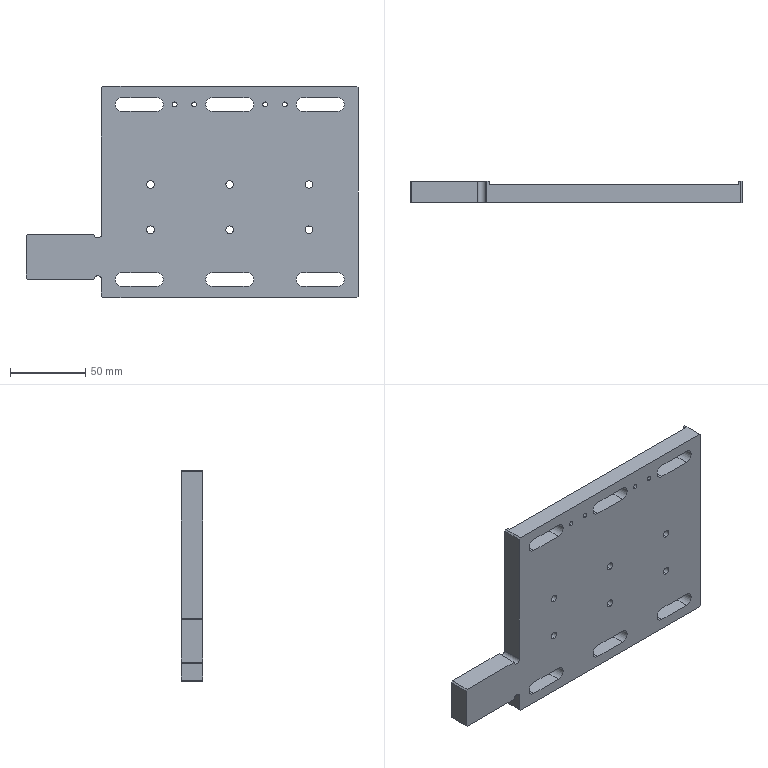Part | SolidWorks | features HoleWzd 3, ICE 3, Chamfer 1, Extrusion 1 | 1 solid | 67 faces | box 220 x 14 x 140 mm | volume 286346 mm3 | cylinder 35 | plane 32 | commonest cylinder face diameters 5 x15 9 x12 3.3 x8